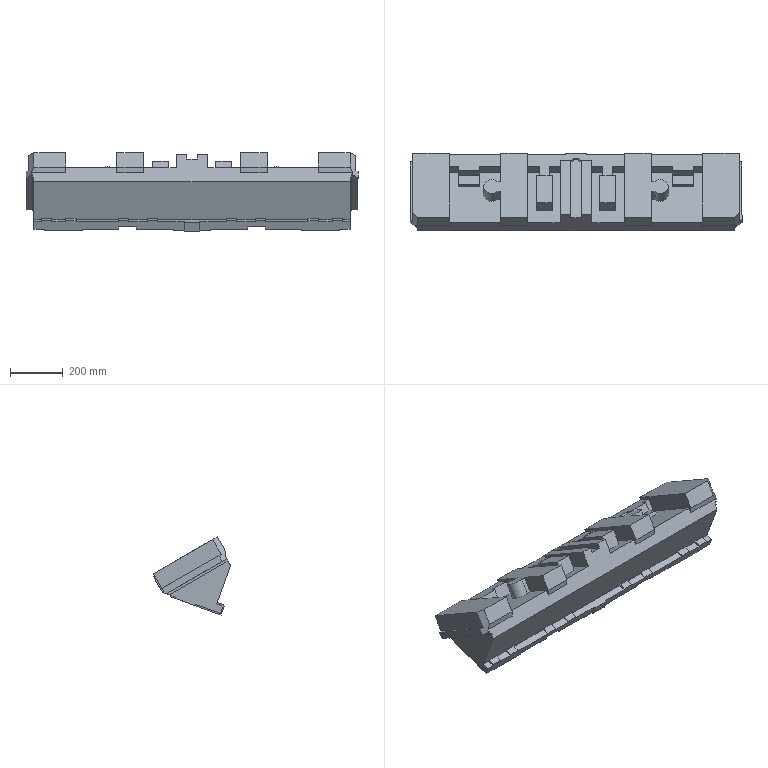Part | NX | features solid 2 | 1 solid | 195 faces | box 1260 x 293.444 x 296.647 mm | volume 46966817 mm3 | plane 177 | cylinder 11 | spline 7 | commonest cylinder face diameters 60 x6 20 x4 40 x1